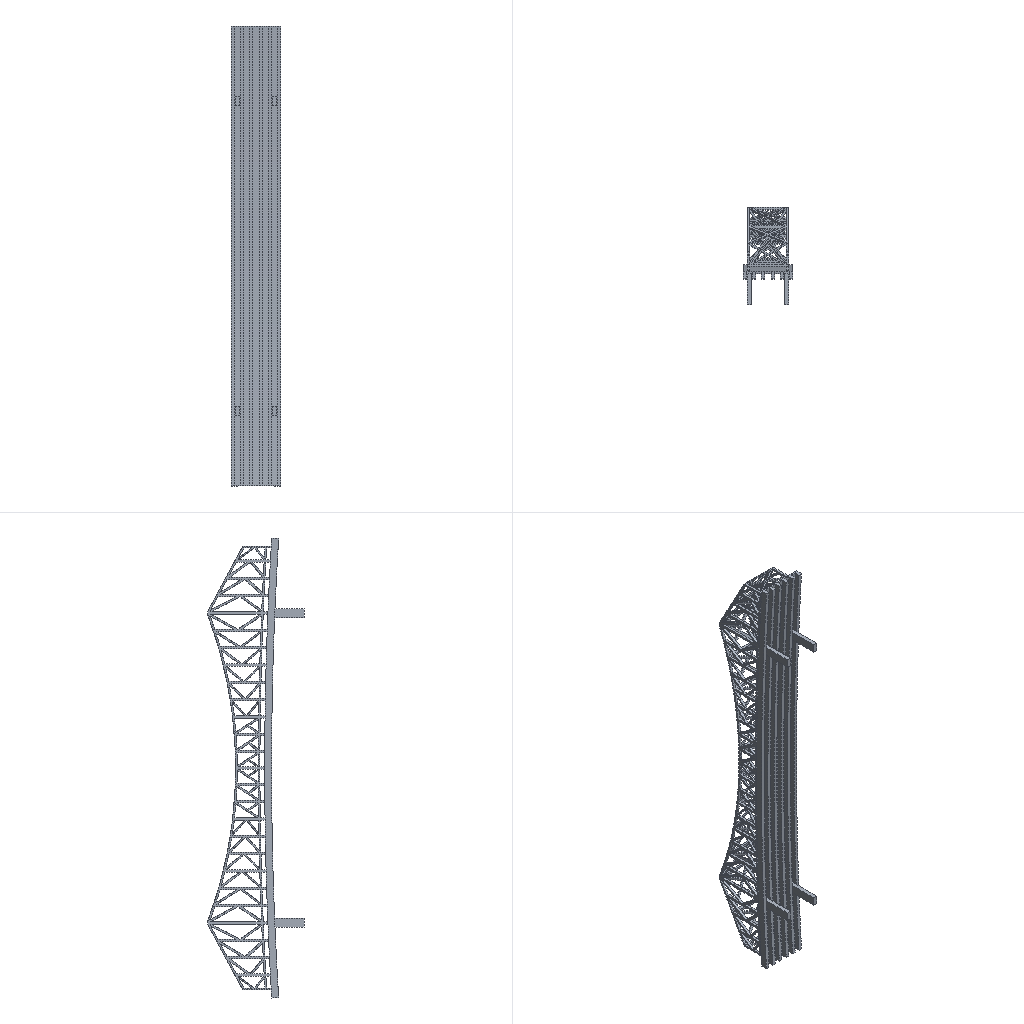Simulation study | ansys workbench
Set-up summary:
category,name,step,type,value,unit,region
solver,ansys_workbench
units,SI m-kg-s (Pa),,stated,"/units,MKS"
analysis,LS1,,static
load_step,LS1,LS1,static,nsubst=1; time=1
mesh,nodes,,,508695
mesh,elements,,,286282
element_type,SOLID187,,,269713
element_type,SURF154,,,13912
element_type,TARGE170,,,1118
element_type,CONTA174,,,1118
element_type,SOLID186,,,421
material,Structural Steel,,E,2e+11,Pa
material,Structural Steel,,nu,0.3
material,Structural Steel,,density,7850,kg m^-3
material,Structural Steel,,conductivity,60.5,W m^-1 C^-1
material,Structural Steel,,specific_heat,434,J kg^-1 C^-1
material,Structural Steel,,cte,1.2e-05,C^-1
material,Structural Steel,,permeability,10000
material,Structural Steel,,resistivity,1.7e-07,kg m^3 A^-2 s^-3
load,Define Force Using Surface Effect Elements,LS1,surface-effect pres face 2,-205379,,SURF154 #26
load,Define Force Using Surface Effect Elements,LS1,surface-effect pres face 3,1.37477e-10,,SURF154 #26
bc,Fixed Supports,model,fixed,[dofs=ALL],,_FIXEDSU
contact,Contact Region,,bonded (always),element=CONTA174
contact,Contact Region 2,,bonded (always),element=CONTA174
contact,Contact Region 3,,bonded (always),element=CONTA174
contact,Contact Region 4,,bonded (always),element=CONTA174
contact,Contact Region 5,,bonded (always),element=CONTA174
contact,Contact Region 6,,bonded (always),element=CONTA174
contact,Contact Region 7,,bonded (always),element=CONTA174
contact,Contact Region 8,,bonded (always),element=CONTA174
named_set,_FIXEDSU,,node,2328
Ansys APDL input file, long lists of numbers shortened:
/batch
/config,noeldb,1     ! force off writing results to database
*get,_wallstrt,active,,time,wall
! ANSYS input file written by Workbench version 2024 R2
! File used for geometry attach:
/title,wbnew--____ (A5)
! ****** Begin Custom Load Command Snippet ******
/COM, ACT Extensions:
/COM,     LSDYNA, 2024.2
/COM,/COM,     ANSYSMotion, 2024.2
/COM,
! ****** End   Custom Load Command Snippet ******
*DIM,_wb_ProjectScratch_dir,string,248
_wb_ProjectScratch_dir(1) = ''
*DIM,_wb_SolverFiles_dir,string,248
_wb_SolverFiles_dir(1) = ''
*DIM,_wb_userfiles_dir,string,248
_wb_userfiles_dir(1) = ''
/com,--- Data in consistent MKS units. See Solving Units in the help system for more information.
/units,MKS
/nopr
/wb,file,start              !  signify a WB generated input file
/prep7
! Turn off shape checking because checks already performed inside WB mesher.
! See help system for more information.
SHPP,OFF,,NOWARN
/nolist
etcon,set             ! allow ANSYS to choose best KEYOP's for 180x elements, resets any applicable keyopt to MAPDL defaults
/com,*********** Nodes for the whole assembly ***********
nblock,3,,559564
(1i9,3e20.9e3)
   501944     1.938972592E-02     7.555537585E-02    -1.848417273E-01
! (508694 more lines like these left out)
-1
/wb,elem,start            !  set before creation of elements
/com,*********** Elements for Body 1 'Part 1' ***********
et,1,187
eblock,19,solid,,266677
(19i9)
        1        1        1        1        0        0        0        0       10        0        1    66776    82081    76779    82078   450516   490316   450514   450515
! (533353 more lines like these left out)
-1
/com,*********** Elements for Body 2 'Part 2' ***********
et,2,186
keyo,2,2,1          ! set full integration on SOLID186
eblock,19,solid,,87
(19i9)
        2        2        2        2        0        0        0        0       20        0   266678   497557   497558   497711   497710   497560   497559   497685   497686
! (173 more lines like these left out)
-1
/com,*********** Elements for Body 3 'Part 3' ***********
et,3,187
eblock,19,solid,,745
(19i9)
        3        3        3        3        0        0        0        0       10        0   266765   498503   498735   498516   498722   499304   499381   499300   499303
! (1489 more lines like these left out)
-1
/com,*********** Elements for Body 4 'Part 4' ***********
et,4,187
eblock,19,solid,,766
(19i9)
        4        4        4        4        0        0        0        0       10        0   267510   500323   500454   500401   500481   501509   501801   501508   501511
! (1531 more lines like these left out)
-1
/com,*********** Elements for Body 5 'Part 5' ***********
et,5,186
keyo,5,2,1          ! set full integration on SOLID186
eblock,19,solid,,115
(19i9)
        5        5        5        5        0        0        0        0       20        0   268276   501956   502220   502221   501985   502045   502126   502125   502016
! (229 more lines like these left out)
-1
/com,*********** Elements for Body 6 'Part 6' ***********
et,6,186
keyo,6,2,1          ! set full integration on SOLID186
eblock,19,solid,,103
(19i9)
        6        6        6        6        0        0        0        0       20        0   268391   503067   503068   503327   503326   503104   503103   503158   503159
! (205 more lines like these left out)
-1
/com,*********** Elements for Body 7 'Part 7' ***********
et,7,187
eblock,19,solid,,745
(19i9)
        7        7        7        7        0        0        0        0       10        0   268494   504057   504362   504058   504060   504535   504539   504528   504530
! (1489 more lines like these left out)
-1
/com,*********** Elements for Body 8 'Part 8' ***********
et,8,187
eblock,19,solid,,780
(19i9)
        8        8        8        8        0        0        0        0       10        0   269239   505961   506090   506036   506111   507174   507474   507172   507176
! (1559 more lines like these left out)
-1
/com,*********** Elements for Body 9 'Part 9' ***********
et,9,186
keyo,9,2,1          ! set full integration on SOLID186
eblock,19,solid,,116
(19i9)
        9        9        9        9        0        0        0        0       20        0   270019   507613   507649   507627   507864   507686   507650   507672   507798
! (231 more lines like these left out)
-1
/wb,elem,end               !  done creating elements
/com,*********** Send User Defined Coordinate System(s) ***********
csys,0
toffst,273.15,      ! Temperature offset from absolute zero
/com,*********** Set Reference Temperature ***********
tref,22.
/wb,mat,start              !  starting to send materials
/com,*********** Send Materials ***********
Temperature = 'TEMP' ! Temperature
MP,DENS,1,7850,	! kg m^-3
MP,ALPX,1,1.2e-05,	! C^-1
MP,C,1,434,	! J kg^-1 C^-1
MP,KXX,1,60.5,	! W m^-1 C^-1
MP,RSVX,1,1.7e-07,	! kg m^3 A^-2 s^-3
MP,EX,1,200000000000,	! Pa
MP,NUXY,1,0.3,
MP,MURX,1,10000,
Temperature = 'TEMP' ! Temperature
MP,DENS,2,7850,	! kg m^-3
MP,ALPX,2,1.2e-05,	! C^-1
MP,C,2,434,	! J kg^-1 C^-1
MP,KXX,2,60.5,	! W m^-1 C^-1
MP,RSVX,2,1.7e-07,	! kg m^3 A^-2 s^-3
MP,EX,2,200000000000,	! Pa
MP,NUXY,2,0.3,
MP,MURX,2,10000,
Temperature = 'TEMP' ! Temperature
MP,DENS,3,7850,	! kg m^-3
MP,ALPX,3,1.2e-05,	! C^-1
MP,C,3,434,	! J kg^-1 C^-1
MP,KXX,3,60.5,	! W m^-1 C^-1
MP,RSVX,3,1.7e-07,	! kg m^3 A^-2 s^-3
MP,EX,3,200000000000,	! Pa
MP,NUXY,3,0.3,
MP,MURX,3,10000,
Temperature = 'TEMP' ! Temperature
MP,DENS,4,7850,	! kg m^-3
MP,ALPX,4,1.2e-05,	! C^-1
MP,C,4,434,	! J kg^-1 C^-1
MP,KXX,4,60.5,	! W m^-1 C^-1
MP,RSVX,4,1.7e-07,	! kg m^3 A^-2 s^-3
MP,EX,4,200000000000,	! Pa
MP,NUXY,4,0.3,
MP,MURX,4,10000,
Temperature = 'TEMP' ! Temperature
MP,DENS,5,7850,	! kg m^-3
MP,ALPX,5,1.2e-05,	! C^-1
MP,C,5,434,	! J kg^-1 C^-1
MP,KXX,5,60.5,	! W m^-1 C^-1
MP,RSVX,5,1.7e-07,	! kg m^3 A^-2 s^-3
MP,EX,5,200000000000,	! Pa
MP,NUXY,5,0.3,
MP,MURX,5,10000,
Temperature = 'TEMP' ! Temperature
MP,DENS,6,7850,	! kg m^-3
MP,ALPX,6,1.2e-05,	! C^-1
MP,C,6,434,	! J kg^-1 C^-1
MP,KXX,6,60.5,	! W m^-1 C^-1
MP,RSVX,6,1.7e-07,	! kg m^3 A^-2 s^-3
MP,EX,6,200000000000,	! Pa
MP,NUXY,6,0.3,
MP,MURX,6,10000,
Temperature = 'TEMP' ! Temperature
MP,DENS,7,7850,	! kg m^-3
MP,ALPX,7,1.2e-05,	! C^-1
MP,C,7,434,	! J kg^-1 C^-1
MP,KXX,7,60.5,	! W m^-1 C^-1
MP,RSVX,7,1.7e-07,	! kg m^3 A^-2 s^-3
MP,EX,7,200000000000,	! Pa
MP,NUXY,7,0.3,
MP,MURX,7,10000,
Temperature = 'TEMP' ! Temperature
MP,DENS,8,7850,	! kg m^-3
MP,ALPX,8,1.2e-05,	! C^-1
MP,C,8,434,	! J kg^-1 C^-1
MP,KXX,8,60.5,	! W m^-1 C^-1
MP,RSVX,8,1.7e-07,	! kg m^3 A^-2 s^-3
MP,EX,8,200000000000,	! Pa
MP,NUXY,8,0.3,
MP,MURX,8,10000,
Temperature = 'TEMP' ! Temperature
MP,DENS,9,7850,	! kg m^-3
MP,ALPX,9,1.2e-05,	! C^-1
MP,C,9,434,	! J kg^-1 C^-1
MP,KXX,9,60.5,	! W m^-1 C^-1
MP,RSVX,9,1.7e-07,	! kg m^3 A^-2 s^-3
MP,EX,9,200000000000,	! Pa
MP,NUXY,9,0.3,
MP,MURX,9,10000,
/wb,mat,end                !  done sending materials
!************************* Model Summary ********************
!Part 1,	ç»æé¢,	matid,	1
!Part 2,	ç»æé¢,	matid,	2
!Part 3,	ç»æé¢,	matid,	3
!Part 4,	ç»æé¢,	matid,	4
!Part 5,	ç»æé¢,	matid,	5
!Part 6,	ç»æé¢,	matid,	6
!Part 7,	ç»æé¢,	matid,	7
!Part 8,	ç»æé¢,	matid,	8
!Part 9,	ç»æé¢,	matid,	9
!************************* End Model Summary ********************
! get the diagonal of the bounding box. Needed later for other things
*get,_xmin,node,,mnloc,x
*get,_ymin,node,,mnloc,y
*get,_zmin,node,,mnloc,z
*get,_xmax,node,,mxloc,x
*get,_ymax,node,,mxloc,y
*get,_zmax,node,,mxloc,z
_ASMDIAG=(_xmax-_xmin)*(_xmax-_xmin)+(_ymax-_ymin)*(_ymax-_ymin)+(_zmax-_zmin)*(_zmax-_zmin)
_ASMDIAG=SQRT(_ASMDIAG)
/wb,contact,start          !  starting to send contact
/com,*********** Create Contact "½Ó´¥ÇøÓò" ***********
/com,            Real Constant Set For Above Contact Is 11 & 10
*set,tid,11
*set,cid,10
r,tid
r,cid
et,tid,170
et,cid,174
eblock,10,,,149
(15i9)
   406715       11       11       11        0     2713     2714     2843     2843    99135    99143     2843    99136
! (148 more lines like these left out)
-1
eblock,10,,,149
(15i9)
   406864       10       10       10        0     2713     2714     2843     2843    99135    99143     2843    99136
! (148 more lines like these left out)
-1
eblock,10,,,8
(15i9)
   407013       10       11       10        0   497727   497728   497670   497669   498300   498214   498211   498213
! (7 more lines like these left out)
-1
eblock,10,,,8
(15i9)
   407021       11       10       11        0   497727   497728   497670   497669   498300   498214   498211   498213
! (7 more lines like these left out)
-1
keyo,cid,8,2               ! auto create asymmetric contact (from Program Controlled setting)
keyo,cid,10,0              ! adjust contact stiffness each NR iteration (from Program Controlled setting)
keyo,cid,12,5              ! bonded always
keyo,cid,18,1              ! small sliding turned on by application
keyo,cid,2,2               ! MPC for bonded contacts (from Program Controlled setting)
keyo,tid,5,0               ! Automatic constraint type detection
keyo,cid,4,2               ! on nodal point - normal to target surface (from Program Controlled setting)
keyo,cid,9,1               ! ignore initial gaps/penetration
keyo,cid,7,0               ! No Prediction
rmod,tid,3,10.      ! FKN
rmod,tid,5,0.       ! ICONT
rmod,tid,6,0.       ! PINB
rmod,tid,10,0.      ! CNOF
rmod,tid,12,0.      ! FKT
rmod,tid,36,56      ! WB DSID
rmod,cid,3,10.      ! FKN
rmod,cid,5,0.       ! ICONT
rmod,cid,6,0.       ! PINB
rmod,cid,10,0.      ! CNOF
rmod,cid,12,0.      ! FKT
rmod,cid,36,56      ! WB DSID
/com,*********** Create Contact "½Ó´¥ÇøÓò 2" ***********
/com,            Real Constant Set For Above Contact Is 13 & 12
*set,tid,13
*set,cid,12
r,tid
r,cid
et,tid,170
et,cid,174
eblock,10,,,142
(15i9)
   407029       13       13       13        0     2880     2899     3102     3102   100099   100247     3102   100101
! (141 more lines like these left out)
-1
eblock,10,,,142
(15i9)
   407171       12       12       12        0     2880     2899     3102     3102   100099   100247     3102   100101
! (141 more lines like these left out)
-1
eblock,10,,,17
(15i9)
   407313       12       13       12        0   498459   498464   498460   498460   499061   499065   498460   499058
! (16 more lines like these left out)
-1
eblock,10,,,17
(15i9)
   407330       13       12       13        0   498459   498464   498460   498460   499061   499065   498460   499058
! (16 more lines like these left out)
-1
keyo,cid,8,2               ! auto create asymmetric contact (from Program Controlled setting)
keyo,cid,10,0              ! adjust contact stiffness each NR iteration (from Program Controlled setting)
keyo,cid,12,5              ! bonded always
keyo,cid,18,1              ! small sliding turned on by application
keyo,cid,2,2               ! MPC for bonded contacts (from Program Controlled setting)
keyo,tid,5,0               ! Automatic constraint type detection
keyo,cid,4,2               ! on nodal point - normal to target surface (from Program Controlled setting)
keyo,cid,9,1               ! ignore initial gaps/penetration
keyo,cid,7,0               ! No Prediction
rmod,tid,3,10.      ! FKN
rmod,tid,5,0.       ! ICONT
rmod,tid,6,0.       ! PINB
rmod,tid,10,0.      ! CNOF
rmod,tid,12,0.      ! FKT
rmod,tid,36,59      ! WB DSID
rmod,cid,3,10.      ! FKN
rmod,cid,5,0.       ! ICONT
rmod,cid,6,0.       ! PINB
rmod,cid,10,0.      ! CNOF
rmod,cid,12,0.      ! FKT
rmod,cid,36,59      ! WB DSID
/com,*********** Create Contact "½Ó´¥ÇøÓò 3" ***********
/com,            Real Constant Set For Above Contact Is 15 & 14
*set,tid,15
*set,cid,14
r,tid
r,cid
et,tid,170
et,cid,174
eblock,10,,,149
(15i9)
   407347       15       15       15        0     3539     3540    37958    37958   104155   104162    37958   104156
! (148 more lines like these left out)
-1
eblock,10,,,149
(15i9)
   407496       14       14       14        0     3539     3540    37958    37958   104155   104162    37958   104156
! (148 more lines like these left out)
-1
eblock,10,,,20
(15i9)
   407645       14       15       14        0   500134   500192   500191   500191   500497   500796   500191   500496
! (19 more lines like these left out)
-1
eblock,10,,,20
(15i9)
   407665       15       14       15        0   500134   500192   500191   500191   500497   500796   500191   500496
! (19 more lines like these left out)
-1
keyo,cid,8,2               ! auto create asymmetric contact (from Program Controlled setting)
keyo,cid,10,0              ! adjust contact stiffness each NR iteration (from Program Controlled setting)
keyo,cid,12,5              ! bonded always
keyo,cid,18,1              ! small sliding turned on by application
keyo,cid,2,2               ! MPC for bonded contacts (from Program Controlled setting)
keyo,tid,5,0               ! Automatic constraint type detection
keyo,cid,4,2               ! on nodal point - normal to target surface (from Program Controlled setting)
keyo,cid,9,1               ! ignore initial gaps/penetration
keyo,cid,7,0               ! No Prediction
rmod,tid,3,10.      ! FKN
rmod,tid,5,0.       ! ICONT
rmod,tid,6,0.       ! PINB
rmod,tid,10,0.      ! CNOF
rmod,tid,12,0.      ! FKT
rmod,tid,36,62      ! WB DSID
rmod,cid,3,10.      ! FKN
rmod,cid,5,0.       ! ICONT
rmod,cid,6,0.       ! PINB
rmod,cid,10,0.      ! CNOF
rmod,cid,12,0.      ! FKT
rmod,cid,36,62      ! WB DSID
/com,*********** Create Contact "½Ó´¥ÇøÓò 4" ***********
/com,            Real Constant Set For Above Contact Is 17 & 16
*set,tid,17
*set,cid,16
r,tid
r,cid
et,tid,170
et,cid,174
eblock,10,,,68
(15i9)
   407685       17       17       17        0     3952    29760     4243     4243   106619   108341     4243   106618
! (67 more lines like these left out)
-1
eblock,10,,,68
(15i9)
   407753       16       16       16        0     3952    29760     4243     4243   106619   108341     4243   106618
! (67 more lines like these left out)
-1
eblock,10,,,6
(15i9)
   407821       16       17       16        0   502205   502206   502142   502141   502955   502861   502859   502860
   407822       16       17       16        0   502265   502095   502144   502204   502768   502767   502865   502954
   407823       16       17       16        0   502211   502209   502137   502136   502961   502853   502850   502851
   407824       16       17       16        0   502209   502210   502138   502137   502960   502854   502852   502853
   407825       16       17       16        0   502145   502069   502278   502201   502712   502714   502951   502867
   407826       16       17       16        0   502069   502173   502186   502278   502713   502920   502934   502714
-1
eblock,10,,,6
(15i9)
   407827       17       16       17        0   502205   502206   502142   502141   502955   502861   502859   502860
   407828       17       16       17        0   502265   502095   502144   502204   502768   502767   502865   502954
   407829       17       16       17        0   502211   502209   502137   502136   502961   502853   502850   502851
   407830       17       16       17        0   502209   502210   502138   502137   502960   502854   502852   502853
   407831       17       16       17        0   502145   502069   502278   502201   502712   502714   502951   502867
   407832       17       16       17        0   502069   502173   502186   502278   502713   502920   502934   502714
-1
keyo,cid,8,2               ! auto create asymmetric contact (from Program Controlled setting)
keyo,cid,10,0              ! adjust contact stiffness each NR iteration (from Program Controlled setting)
keyo,cid,12,5              ! bonded always
keyo,cid,18,1              ! small sliding turned on by application
keyo,cid,2,2               ! MPC for bonded contacts (from Program Controlled setting)
keyo,tid,5,0               ! Automatic constraint type detection
keyo,cid,4,2               ! on nodal point - normal to target surface (from Program Controlled setting)
keyo,cid,9,1               ! ignore initial gaps/penetration
keyo,cid,7,0               ! No Prediction
rmod,tid,3,10.      ! FKN
rmod,tid,5,0.       ! ICONT
rmod,tid,6,0.       ! PINB
rmod,tid,10,0.      ! CNOF
rmod,tid,12,0.      ! FKT
rmod,tid,36,65      ! WB DSID
rmod,cid,3,10.      ! FKN
rmod,cid,5,0.       ! ICONT
rmod,cid,6,0.       ! PINB
rmod,cid,10,0.      ! CNOF
rmod,cid,12,0.      ! FKT
rmod,cid,36,65      ! WB DSID
/com,*********** Create Contact "½Ó´¥ÇøÓò 5" ***********
/com,            Real Constant Set For Above Contact Is 19 & 18
*set,tid,19
*set,cid,18
r,tid
r,cid
et,tid,170
et,cid,174
eblock,10,,,149
(15i9)
   407833       19       19       19        0     6077     8513     8515     8515   119440   134163     8515   119441
! (148 more lines like these left out)
-1
eblock,10,,,149
(15i9)
   407982       18       18       18        0     6077     8513     8515     8515   119440   134163     8515   119441
! (148 more lines like these left out)
-1
eblock,10,,,8
(15i9)
   408131       18       19       18        0   503257   503256   503242   503228   503926   503911   503883   503884
! (7 more lines like these left out)
-1
eblock,10,,,8
(15i9)
   408139       19       18       19        0   503257   503256   503242   503228   503926   503911   503883   503884
! (7 more lines like these left out)
-1
keyo,cid,8,2               ! auto create asymmetric contact (from Program Controlled setting)
keyo,cid,10,0              ! adjust contact stiffness each NR iteration (from Program Controlled setting)
keyo,cid,12,5              ! bonded always
keyo,cid,18,1              ! small sliding turned on by application
keyo,cid,2,2               ! MPC for bonded contacts (from Program Controlled setting)
keyo,tid,5,0               ! Automatic constraint type detection
keyo,cid,4,2               ! on nodal point - normal to target surface (from Program Controlled setting)
keyo,cid,9,1               ! ignore initial gaps/penetration
keyo,cid,7,0               ! No Prediction
rmod,tid,3,10.      ! FKN
rmod,tid,5,0.       ! ICONT
rmod,tid,6,0.       ! PINB
rmod,tid,10,0.      ! CNOF
rmod,tid,12,0.      ! FKT
rmod,tid,36,68      ! WB DSID
rmod,cid,3,10.      ! FKN
rmod,cid,5,0.       ! ICONT
rmod,cid,6,0.       ! PINB
rmod,cid,10,0.      ! CNOF
rmod,cid,12,0.      ! FKT
rmod,cid,36,68      ! WB DSID
/com,*********** Create Contact "½Ó´¥ÇøÓò 6" ***********
/com,            Real Constant Set For Above Contact Is 21 & 20
*set,tid,21
*set,cid,20
r,tid
r,cid
et,tid,170
et,cid,174
eblock,10,,,142
(15i9)
   408147       21       21       21        0     6101    29753     7288     7288   119602   126846     7288   119600
! (141 more lines like these left out)
-1
eblock,10,,,142
(15i9)
   408289       20       20       20        0     6101    29753     7288     7288   119602   126846     7288   119600
! (141 more lines like these left out)
-1
eblock,10,,,17
(15i9)
   408431       20       21       20        0   504052   504054   504053   504053   504513   504515   504053   504512
! (16 more lines like these left out)
-1
eblock,10,,,17
(15i9)
   408448       21       20       21        0   504052   504054   504053   504053   504513   504515   504053   504512
! (16 more lines like these left out)
-1
keyo,cid,8,2               ! auto create asymmetric contact (from Program Controlled setting)
keyo,cid,10,0              ! adjust contact stiffness each NR iteration (from Program Controlled setting)
keyo,cid,12,5              ! bonded always
keyo,cid,18,1              ! small sliding turned on by application
keyo,cid,2,2               ! MPC for bonded contacts (from Program Controlled setting)
keyo,tid,5,0               ! Automatic constraint type detection
keyo,cid,4,2               ! on nodal point - normal to target surface (from Program Controlled setting)
keyo,cid,9,1               ! ignore initial gaps/penetration
keyo,cid,7,0               ! No Prediction
rmod,tid,3,10.      ! FKN
rmod,tid,5,0.       ! ICONT
rmod,tid,6,0.       ! PINB
rmod,tid,10,0.      ! CNOF
rmod,tid,12,0.      ! FKT
rmod,tid,36,71      ! WB DSID
rmod,cid,3,10.      ! FKN
rmod,cid,5,0.       ! ICONT
rmod,cid,6,0.       ! PINB
rmod,cid,10,0.      ! CNOF
rmod,cid,12,0.      ! FKT
rmod,cid,36,71      ! WB DSID
/com,*********** Create Contact "½Ó´¥ÇøÓò 7" ***********
/com,            Real Constant Set For Above Contact Is 23 & 22
*set,tid,23
*set,cid,22
r,tid
r,cid
et,tid,170
et,cid,174
eblock,10,,,149
(15i9)
   408465       23       23       23        0     6101    29753     7288     7288   119602   126846     7288   119600
! (148 more lines like these left out)
-1
eblock,10,,,149
(15i9)
   408614       22       22       22        0     6101    29753     7288     7288   119602   126846     7288   119600
! (148 more lines like these left out)
-1
eblock,10,,,20
(15i9)
   408763       22       23       22        0   505796   505863   505862   505862   506307   506652   505862   506306
! (19 more lines like these left out)
-1
eblock,10,,,20
(15i9)
   408783       23       22       23        0   505796   505863   505862   505862   506307   506652   505862   506306
! (19 more lines like these left out)
-1
keyo,cid,8,2               ! auto create asymmetric contact (from Program Controlled setting)
keyo,cid,10,0              ! adjust contact stiffness each NR iteration (from Program Controlled setting)
keyo,cid,12,5              ! bonded always
keyo,cid,18,1              ! small sliding turned on by application
keyo,cid,2,2               ! MPC for bonded contacts (from Program Controlled setting)
keyo,tid,5,0               ! Automatic constraint type detection
keyo,cid,4,2               ! on nodal point - normal to target surface (from Program Controlled setting)
keyo,cid,9,1               ! ignore initial gaps/penetration
keyo,cid,7,0               ! No Prediction
rmod,tid,3,10.      ! FKN
rmod,tid,5,0.       ! ICONT
rmod,tid,6,0.       ! PINB
rmod,tid,10,0.      ! CNOF
rmod,tid,12,0.      ! FKT
rmod,tid,36,74      ! WB DSID
rmod,cid,3,10.      ! FKN
rmod,cid,5,0.       ! ICONT
rmod,cid,6,0.       ! PINB
rmod,cid,10,0.      ! CNOF
rmod,cid,12,0.      ! FKT
rmod,cid,36,74      ! WB DSID
/com,*********** Create Contact "½Ó´¥ÇøÓò 8" ***********
/com,            Real Constant Set For Above Contact Is 25 & 24
*set,tid,25
*set,cid,24
r,tid
r,cid
et,tid,170
et,cid,174
eblock,10,,,68
(15i9)
   408803       25       25       25        0     6124     8034     8035     8035   119741   131436     8035   119742
! (67 more lines like these left out)
-1
eblock,10,,,68
(15i9)
   408871       24       24       24        0     6124     8034     8035     8035   119741   131436     8035   119742
! (67 more lines like these left out)
-1
eblock,10,,,6
(15i9)
   408939       24       25       24        0   507734   507915   507828   507822   508401   508585   508576   508400
   408940       24       25       24        0   507758   507891   507890   507771   508452   508650   508477   508450
   408941       24       25       24        0   507823   507826   507891   507758   508578   508582   508452   508451
   408942       24       25       24        0   507819   507831   507830   507818   508571   508587   508570   508569
   408943       24       25       24        0   507814   507834   507835   507813   508563   508592   508561   508560
   408944       24       25       24        0   507815   507836   507834   507814   508564   508593   508563   508562
-1
eblock,10,,,6
(15i9)
   408945       25       24       25        0   507734   507915   507828   507822   508401   508585   508576   508400
   408946       25       24       25        0   507758   507891   507890   507771   508452   508650   508477   508450
   408947       25       24       25        0   507823   507826   507891   507758   508578   508582   508452   508451
   408948       25       24       25        0   507819   507831   507830   507818   508571   508587   508570   508569
   408949       25       24       25        0   507814   507834   507835   507813   508563   508592   508561   508560
   408950       25       24       25        0   507815   507836   507834   507814   508564   508593   508563   508562
-1
keyo,cid,8,2               ! auto create asymmetric contact (from Program Controlled setting)
keyo,cid,10,0              ! adjust contact stiffness each NR iteration (from Program Controlled setting)
keyo,cid,12,5              ! bonded always
keyo,cid,18,1              ! small sliding turned on by application
keyo,cid,2,2               ! MPC for bonded contacts (from Program Controlled setting)
keyo,tid,5,0               ! Automatic constraint type detection
keyo,cid,4,2               ! on nodal point - normal to target surface (from Program Controlled setting)
keyo,cid,9,1               ! ignore initial gaps/penetration
keyo,cid,7,0               ! No Prediction
rmod,tid,3,10.      ! FKN
rmod,tid,5,0.       ! ICONT
rmod,tid,6,0.       ! PINB
rmod,tid,10,0.      ! CNOF
rmod,tid,12,0.      ! FKT
rmod,tid,36,77      ! WB DSID
rmod,cid,3,10.      ! FKN
rmod,cid,5,0.       ! ICONT
rmod,cid,6,0.       ! PINB
rmod,cid,10,0.      ! CNOF
rmod,cid,12,0.      ! FKT
rmod,cid,36,77      ! WB DSID
nsel,all
esel,all
/wb,contact,end            !  done creating contacts
/golist
/wb,load,start             !  starting to send loads
/com,*********** Fixed Supports ***********
CMBLOCK,_FIXEDSU,NODE,     2328
(8i10)
     13380     13389     13392     13393     13394     13395     13396     13962
! (290 more lines like these left out)
cmsel,s,_FIXEDSU
d,all,all
nsel,all
/com,*********** Define Force Using Surface Effect Elements ***********
local,12,0,0.,0.,0.,0.,0.,0.
csys,0
et,26,154
mat,26
eblock,10,,,13912
(15i9)
   408951       26       26       26       12    20923    20922    38979    38979   222412   222414    38979   222418
! (13911 more lines like these left out)
-1
esel,s,type,,26
keyop,26,2,1        ! Apply load in local coordinate system
keyop,26,7,1        ! Use original area so load is constant in large deformation
esel,all
/gst,on,on
fini
*get,_numnode,node,0,count
*get,_numelem,elem,0,count
*get, _MAXELEMNUM, elem, 0, NUM, MAX
*get, _MAXNODENUM, node, 0, NUM, MAX
*get, _MAXELEMTYPE, etyp, 0, NUM, MAX
*get, _MAXREALCONST, rcon, 0, NUM, MAX
/go
/wb,load,end               !  done creating loads
/com,--- Number of total nodes = %_numnode%
/com,--- Number of contact elements = 16148
/com,--- Number of spring elements = 0
/com,--- Number of bearing elements = 0
/com,--- Number of solid elements = 270134
/com,--- Number of condensed parts = 0
/com,--- Number of total elements = %_numelem%
*get,_wallbsol,active,,time,wall
/com,****************************************************************************
/com,*************************    SOLUTION       ********************************
/com,****************************************************************************
/solu
antype,0                   ! static analysis
_thickRatio=0.111   ! Ratio of thick parts in the model
eqsl,sparse,,,,,1
cntr,print,1               ! print out contact info and also make no initial contact an error
dmpoption,emat,no             ! Don't combine emat file for DANSYS
dmpoption,esav,no             ! Don't combine esav file for DANSYS
nldiag,cont,iter           ! print out contact info each equilibrium iteration
rescontrol,,none                 ! Do not keep any restart files
/com,****************************************************
/com,******************* SOLVE FOR LS 1 OF 1 ****************
esel,s,type,,26
nsle
sfe,all,1,pres,1,0.
sfe,all,2,pres,1,-205379.336
sfe,all,3,pres,1,1.37477149637281e-010
nsel,all
esel,all
/nopr
/gopr
nsub,1,1,1
time,1.
outres,erase
outres,all,none
outres,nsol,all,
outres,rsol,all
outres,eangl,all
outres,etmp,all
outres,veng,all
outres,strs,all,
outres,epel,all,
outres,eppl,all,
outres,cont,all,
! *********** WB SOLVE COMMAND ***********
! check interactive state
*get,ANSINTER_,active,,int
*if,ANSINTER_,ne,0,then
/eof
*endif
solve
/com *************** Write FE CONNECTORS *********
CEWRITE,file,ce,,INTE
/com,****************************************************
/com,*************** FINISHED SOLVE FOR LS 1 *************
*get,_wallasol,active,,time,wall
/nopr
*get,_numnode,node,0,count
*get,_numelem,elem,0,count
*get, _MAXELEMNUM, elem, 0, NUM, MAX
*get, _MAXNODENUM, node, 0, NUM, MAX,,,INTERNAL
*get, _MAXELEMTYPE, etyp, 0, NUM, MAX
*get, _MAXREALCONST, rcon, 0, NUM, MAX
*get,_NSOLTHREADS,active,0,ntfs
*get,_NSOLPROCESSES,active,0,npfs
/gopr
/post1
xmlo,ENCODING,ISO-8859-1
xmlo,parm
/xml,parm,xml
fini
/gopr
*get,_walldone,active,,time,wall
_preptime=(_wallbsol-_wallstrt)*3600
_solvtime=(_wallasol-_wallbsol)*3600
_posttime=(_walldone-_wallasol)*3600
_totaltim=(_walldone-_wallstrt)*3600
*get,_dlbratio,active,0,solu,dlbr
*get,_combtime,active,0,solu,comb
*get,_ssmode,active,0,solu,ssmm
*get,_ndofs,active,0,solu,ndof
*get,_sol_end_time,active,0,set,time
*if,_sol_end_time,eq,1.,then
/fclean				!clean distributed files
*endif
/com,--- Total number of nodes = %_numnode%
/com,--- Total number of elements = %_numelem%
/com,--- Element load balance ratio = %_dlbratio%
/com,--- Time to combine distributed files = %_combtime%
/com,--- Sparse memory mode = %_ssmode%
/com,--- Number of DOF = %_ndofs%
/wb,file,end               ! done with WB generated input
Results summary:
result,analyses[0].index,,,1
result,analyses[0].system,,,SYS
result,analyses[0].deck,,,deck.dat
result,analyses[0].solve_status,,,completed
result,analyses[0].analysis_type,,,static
result,analyses[0].physics,,,mechanical
result,analyses[0].unit_system,,,"MKS: m, kg, N, s, V, A, degC"
result,analyses[0].n_sets,,,1
result,analyses[0].load_steps[0].set,set=1,,1
result,analyses[0].load_steps[0].time_or_freq,set=1,,1
result,analyses[0].load_steps[0].max_displacement_magnitude,set=1,,0.0005485
result,analyses[0].load_steps[0].max_von_mises_nodal,set=1,,3.41257e+08
result,analyses[0].load_steps[0].reaction_force_sum_xyz[1],set=1,,-1.10168e-07
result,analyses[0].load_steps[0].reaction_force_sum_xyz[2],set=1,,5000
result,analyses[0].load_steps[0].reaction_force_sum_xyz[3],set=1,,1.5653e-07